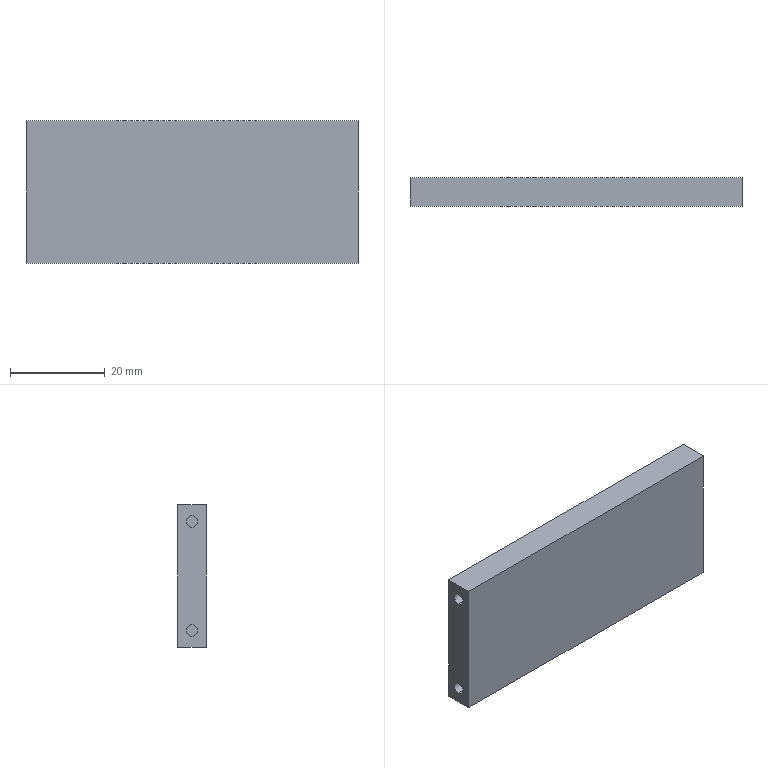Part | SolidWorks | features Cut 2, Extrusion 1 | 1 solid | 18 faces | box 70 x 6 x 30 mm | volume 12502 mm3 | plane 10 | cylinder 8 | commonest cylinder face diameters 2.5 x8
STEP:
#1=CARTESIAN_POINT('',(-30.,3.,-12.75));
#2=VERTEX_POINT('',#1);
#3=CARTESIAN_POINT('',(-30.,3.,-10.25));
#4=VERTEX_POINT('',#3);
#5=CARTESIAN_POINT('',(-30.,3.,-11.5));
#6=DIRECTION('',(-1.,0.,0.));
#7=DIRECTION('',(0.,0.,1.));
#8=AXIS2_PLACEMENT_3D('',#5,#6,#7);
#9=CIRCLE('',#8,1.25);
#10=EDGE_CURVE('',#2,#4,#9,.T.);
#11=ORIENTED_EDGE('',*,*,#10,.F.);
#12=CARTESIAN_POINT('',(-35.,3.,-12.75));
#13=VERTEX_POINT('',#12);
#14=CARTESIAN_POINT('',(-30.,3.,-12.75));
#15=DIRECTION('',(-1.,0.,0.));
#16=VECTOR('',#15,1000.);
#17=LINE('',#14,#16);
#18=EDGE_CURVE('',#2,#13,#17,.T.);
#19=ORIENTED_EDGE('',*,*,#18,.T.);
#20=CARTESIAN_POINT('',(-35.,3.,-10.25));
#21=VERTEX_POINT('',#20);
#22=CARTESIAN_POINT('',(-35.,3.,-11.5));
#23=DIRECTION('',(-1.,0.,0.));
#24=DIRECTION('',(0.,0.,1.));
#25=AXIS2_PLACEMENT_3D('',#22,#23,#24);
#26=CIRCLE('',#25,1.25);
#27=EDGE_CURVE('',#13,#21,#26,.T.);
#28=ORIENTED_EDGE('',*,*,#27,.T.);
#29=CARTESIAN_POINT('',(-30.,3.,-10.25));
#30=DIRECTION('',(-1.,0.,0.));
#31=VECTOR('',#30,1000.);
#32=LINE('',#29,#31);
#33=EDGE_CURVE('',#4,#21,#32,.T.);
#34=ORIENTED_EDGE('',*,*,#33,.F.);
#35=EDGE_LOOP('',(#11,#19,#28,#34));
#36=FACE_OUTER_BOUND('',#35,.T.);
#37=CARTESIAN_POINT('',(-30.,3.,-11.5));
#38=DIRECTION('',(-1.,0.,0.));
#39=DIRECTION('',(0.,0.,1.));
#40=AXIS2_PLACEMENT_3D('',#37,#38,#39);
#41=CYLINDRICAL_SURFACE('',#40,1.25);
#42=ADVANCED_FACE('',(#36),#41,.F.);
#43=CARTESIAN_POINT('',(-30.,3.,10.25));
#44=VERTEX_POINT('',#43);
#45=CARTESIAN_POINT('',(-30.,3.,12.75));
#46=VERTEX_POINT('',#45);
#47=CARTESIAN_POINT('',(-30.,3.,11.5));
#48=DIRECTION('',(-1.,0.,0.));
#49=DIRECTION('',(0.,0.,1.));
#50=AXIS2_PLACEMENT_3D('',#47,#48,#49);
#51=CIRCLE('',#50,1.25);
#52=EDGE_CURVE('',#44,#46,#51,.T.);
#53=ORIENTED_EDGE('',*,*,#52,.F.);
#54=CARTESIAN_POINT('',(-35.,3.,10.25));
#55=VERTEX_POINT('',#54);
#56=CARTESIAN_POINT('',(-30.,3.,10.25));
#57=DIRECTION('',(-1.,0.,0.));
#58=VECTOR('',#57,1000.);
#59=LINE('',#56,#58);
#60=EDGE_CURVE('',#44,#55,#59,.T.);
#61=ORIENTED_EDGE('',*,*,#60,.T.);
#62=CARTESIAN_POINT('',(-35.,3.,12.75));
#63=VERTEX_POINT('',#62);
#64=CARTESIAN_POINT('',(-35.,3.,11.5));
#65=DIRECTION('',(-1.,0.,0.));
#66=DIRECTION('',(0.,0.,1.));
#67=AXIS2_PLACEMENT_3D('',#64,#65,#66);
#68=CIRCLE('',#67,1.25);
#69=EDGE_CURVE('',#55,#63,#68,.T.);
#70=ORIENTED_EDGE('',*,*,#69,.T.);
#71=CARTESIAN_POINT('',(-30.,3.,12.75));
#72=DIRECTION('',(-1.,0.,0.));
#73=VECTOR('',#72,1000.);
#74=LINE('',#71,#73);
#75=EDGE_CURVE('',#46,#63,#74,.T.);
#76=ORIENTED_EDGE('',*,*,#75,.F.);
#77=EDGE_LOOP('',(#53,#61,#70,#76));
#78=FACE_OUTER_BOUND('',#77,.T.);
#79=CARTESIAN_POINT('',(-30.,3.,11.5));
#80=DIRECTION('',(-1.,0.,0.));
#81=DIRECTION('',(0.,0.,1.));
#82=AXIS2_PLACEMENT_3D('',#79,#80,#81);
#83=CYLINDRICAL_SURFACE('',#82,1.25);
#84=ADVANCED_FACE('',(#78),#83,.F.);
#85=CARTESIAN_POINT('',(30.,3.,-10.25));
#86=VERTEX_POINT('',#85);
#87=CARTESIAN_POINT('',(30.,3.,-12.75));
#88=VERTEX_POINT('',#87);
#89=CARTESIAN_POINT('',(30.,3.,-11.5));
#90=DIRECTION('',(1.,0.,0.));
#91=DIRECTION('',(0.,0.,-1.));
#92=AXIS2_PLACEMENT_3D('',#89,#90,#91);
#93=CIRCLE('',#92,1.25);
#94=EDGE_CURVE('',#86,#88,#93,.T.);
#95=ORIENTED_EDGE('',*,*,#94,.F.);
#96=CARTESIAN_POINT('',(35.,3.,-10.25));
#97=VERTEX_POINT('',#96);
#98=CARTESIAN_POINT('',(30.,3.,-10.25));
#99=DIRECTION('',(1.,0.,0.));
#100=VECTOR('',#99,1000.);
#101=LINE('',#98,#100);
#102=EDGE_CURVE('',#86,#97,#101,.T.);
#103=ORIENTED_EDGE('',*,*,#102,.T.);
#104=CARTESIAN_POINT('',(35.,3.,-12.75));
#105=VERTEX_POINT('',#104);
#106=CARTESIAN_POINT('',(35.,3.,-11.5));
#107=DIRECTION('',(1.,0.,0.));
#108=DIRECTION('',(0.,0.,-1.));
#109=AXIS2_PLACEMENT_3D('',#106,#107,#108);
#110=CIRCLE('',#109,1.25);
#111=EDGE_CURVE('',#97,#105,#110,.T.);
#112=ORIENTED_EDGE('',*,*,#111,.T.);
#113=CARTESIAN_POINT('',(30.,3.,-12.75));
#114=DIRECTION('',(1.,0.,0.));
#115=VECTOR('',#114,1000.);
#116=LINE('',#113,#115);
#117=EDGE_CURVE('',#88,#105,#116,.T.);
#118=ORIENTED_EDGE('',*,*,#117,.F.);
#119=EDGE_LOOP('',(#95,#103,#112,#118));
#120=FACE_OUTER_BOUND('',#119,.T.);
#121=CARTESIAN_POINT('',(30.,3.,-11.5));
#122=DIRECTION('',(1.,0.,0.));
#123=DIRECTION('',(0.,0.,-1.));
#124=AXIS2_PLACEMENT_3D('',#121,#122,#123);
#125=CYLINDRICAL_SURFACE('',#124,1.25);
#126=ADVANCED_FACE('',(#120),#125,.F.);
#127=CARTESIAN_POINT('',(30.,3.,12.75));
#128=VERTEX_POINT('',#127);
#129=CARTESIAN_POINT('',(30.,3.,10.25));
#130=VERTEX_POINT('',#129);
#131=CARTESIAN_POINT('',(30.,3.,11.5));
#132=DIRECTION('',(1.,0.,0.));
#133=DIRECTION('',(0.,0.,-1.));
#134=AXIS2_PLACEMENT_3D('',#131,#132,#133);
#135=CIRCLE('',#134,1.25);
#136=EDGE_CURVE('',#128,#130,#135,.T.);
#137=ORIENTED_EDGE('',*,*,#136,.F.);
#138=CARTESIAN_POINT('',(35.,3.,12.75));
#139=VERTEX_POINT('',#138);
#140=CARTESIAN_POINT('',(30.,3.,12.75));
#141=DIRECTION('',(1.,0.,0.));
#142=VECTOR('',#141,1000.);
#143=LINE('',#140,#142);
#144=EDGE_CURVE('',#128,#139,#143,.T.);
#145=ORIENTED_EDGE('',*,*,#144,.T.);
#146=CARTESIAN_POINT('',(35.,3.,10.25));
#147=VERTEX_POINT('',#146);
#148=CARTESIAN_POINT('',(35.,3.,11.5));
#149=DIRECTION('',(1.,0.,0.));
#150=DIRECTION('',(0.,0.,-1.));
#151=AXIS2_PLACEMENT_3D('',#148,#149,#150);
#152=CIRCLE('',#151,1.25);
#153=EDGE_CURVE('',#139,#147,#152,.T.);
#154=ORIENTED_EDGE('',*,*,#153,.T.);
#155=CARTESIAN_POINT('',(30.,3.,10.25));
#156=DIRECTION('',(1.,0.,0.));
#157=VECTOR('',#156,1000.);
#158=LINE('',#155,#157);
#159=EDGE_CURVE('',#130,#147,#158,.T.);
#160=ORIENTED_EDGE('',*,*,#159,.F.);
#161=EDGE_LOOP('',(#137,#145,#154,#160));
#162=FACE_OUTER_BOUND('',#161,.T.);
#163=CARTESIAN_POINT('',(30.,3.,11.5));
#164=DIRECTION('',(1.,0.,0.));
#165=DIRECTION('',(0.,0.,-1.));
#166=AXIS2_PLACEMENT_3D('',#163,#164,#165);
#167=CYLINDRICAL_SURFACE('',#166,1.25);
#168=ADVANCED_FACE('',(#162),#167,.F.);
#169=CARTESIAN_POINT('',(35.,3.,-11.5));
#170=DIRECTION('',(1.,0.,0.));
#171=DIRECTION('',(0.,0.,-1.));
#172=AXIS2_PLACEMENT_3D('',#169,#170,#171);
#173=CIRCLE('',#172,1.25);
#174=EDGE_CURVE('',#105,#97,#173,.T.);
#175=ORIENTED_EDGE('',*,*,#174,.F.);
#176=ORIENTED_EDGE('',*,*,#111,.F.);
#177=EDGE_LOOP('',(#175,#176));
#178=FACE_BOUND('',#177,.T.);
#179=CARTESIAN_POINT('',(35.,3.,11.5));
#180=DIRECTION('',(1.,0.,0.));
#181=DIRECTION('',(0.,0.,-1.));
#182=AXIS2_PLACEMENT_3D('',#179,#180,#181);
#183=CIRCLE('',#182,1.25);
#184=EDGE_CURVE('',#147,#139,#183,.T.);
#185=ORIENTED_EDGE('',*,*,#184,.F.);
#186=ORIENTED_EDGE('',*,*,#153,.F.);
#187=EDGE_LOOP('',(#185,#186));
#188=FACE_BOUND('',#187,.T.);
#189=CARTESIAN_POINT('',(35.,0.,15.));
#190=VERTEX_POINT('',#189);
#191=CARTESIAN_POINT('',(35.,0.,-15.));
#192=VERTEX_POINT('',#191);
#193=CARTESIAN_POINT('',(35.,0.,-15.));
#194=DIRECTION('',(0.,0.,-1.));
#195=VECTOR('',#194,1000.);
#196=LINE('',#193,#195);
#197=EDGE_CURVE('',#190,#192,#196,.T.);
#198=ORIENTED_EDGE('',*,*,#197,.T.);
#199=CARTESIAN_POINT('',(35.,6.,-15.));
#200=VERTEX_POINT('',#199);
#201=CARTESIAN_POINT('',(35.,6.,-15.));
#202=DIRECTION('',(0.,-1.,0.));
#203=VECTOR('',#202,1000.);
#204=LINE('',#201,#203);
#205=EDGE_CURVE('',#200,#192,#204,.T.);
#206=ORIENTED_EDGE('',*,*,#205,.F.);
#207=CARTESIAN_POINT('',(35.,6.,15.));
#208=VERTEX_POINT('',#207);
#209=CARTESIAN_POINT('',(35.,6.,-15.));
#210=DIRECTION('',(0.,0.,-1.));
#211=VECTOR('',#210,1000.);
#212=LINE('',#209,#211);
#213=EDGE_CURVE('',#208,#200,#212,.T.);
#214=ORIENTED_EDGE('',*,*,#213,.F.);
#215=CARTESIAN_POINT('',(35.,6.,15.));
#216=DIRECTION('',(0.,-1.,0.));
#217=VECTOR('',#216,1000.);
#218=LINE('',#215,#217);
#219=EDGE_CURVE('',#208,#190,#218,.T.);
#220=ORIENTED_EDGE('',*,*,#219,.T.);
#221=EDGE_LOOP('',(#198,#206,#214,#220));
#222=FACE_OUTER_BOUND('',#221,.T.);
#223=CARTESIAN_POINT('',(35.,6.,-15.));
#224=DIRECTION('',(-1.,0.,0.));
#225=DIRECTION('',(0.,0.,1.));
#226=AXIS2_PLACEMENT_3D('',#223,#224,#225);
#227=PLANE('',#226);
#228=ADVANCED_FACE('',(#178,#188,#222),#227,.F.);
#229=CARTESIAN_POINT('',(-35.,0.,-15.));
#230=VERTEX_POINT('',#229);
#231=CARTESIAN_POINT('',(-35.,0.,-15.));
#232=DIRECTION('',(-1.,0.,0.));
#233=VECTOR('',#232,1000.);
#234=LINE('',#231,#233);
#235=EDGE_CURVE('',#192,#230,#234,.T.);
#236=ORIENTED_EDGE('',*,*,#235,.T.);
#237=CARTESIAN_POINT('',(-35.,6.,-15.));
#238=VERTEX_POINT('',#237);
#239=CARTESIAN_POINT('',(-35.,6.,-15.));
#240=DIRECTION('',(0.,-1.,0.));
#241=VECTOR('',#240,1000.);
#242=LINE('',#239,#241);
#243=EDGE_CURVE('',#238,#230,#242,.T.);
#244=ORIENTED_EDGE('',*,*,#243,.F.);
#245=CARTESIAN_POINT('',(-35.,6.,-15.));
#246=DIRECTION('',(-1.,0.,0.));
#247=VECTOR('',#246,1000.);
#248=LINE('',#245,#247);
#249=EDGE_CURVE('',#200,#238,#248,.T.);
#250=ORIENTED_EDGE('',*,*,#249,.F.);
#251=ORIENTED_EDGE('',*,*,#205,.T.);
#252=EDGE_LOOP('',(#236,#244,#250,#251));
#253=FACE_OUTER_BOUND('',#252,.T.);
#254=CARTESIAN_POINT('',(-35.,6.,-15.));
#255=DIRECTION('',(0.,0.,1.));
#256=DIRECTION('',(1.,0.,0.));
#257=AXIS2_PLACEMENT_3D('',#254,#255,#256);
#258=PLANE('',#257);
#259=ADVANCED_FACE('',(#253),#258,.F.);
#260=CARTESIAN_POINT('',(-35.,3.,-11.5));
#261=DIRECTION('',(-1.,0.,0.));
#262=DIRECTION('',(0.,0.,1.));
#263=AXIS2_PLACEMENT_3D('',#260,#261,#262);
#264=CIRCLE('',#263,1.25);
#265=EDGE_CURVE('',#21,#13,#264,.T.);
#266=ORIENTED_EDGE('',*,*,#265,.F.);
#267=ORIENTED_EDGE('',*,*,#27,.F.);
#268=EDGE_LOOP('',(#266,#267));
#269=FACE_BOUND('',#268,.T.);
#270=CARTESIAN_POINT('',(-35.,3.,11.5));
#271=DIRECTION('',(-1.,0.,0.));
#272=DIRECTION('',(0.,0.,1.));
#273=AXIS2_PLACEMENT_3D('',#270,#271,#272);
#274=CIRCLE('',#273,1.25);
#275=EDGE_CURVE('',#63,#55,#274,.T.);
#276=ORIENTED_EDGE('',*,*,#275,.F.);
#277=ORIENTED_EDGE('',*,*,#69,.F.);
#278=EDGE_LOOP('',(#276,#277));
#279=FACE_BOUND('',#278,.T.);
#280=CARTESIAN_POINT('',(-35.,0.,15.));
#281=VERTEX_POINT('',#280);
#282=CARTESIAN_POINT('',(-35.,0.,-15.));
#283=DIRECTION('',(0.,0.,1.));
#284=VECTOR('',#283,1000.);
#285=LINE('',#282,#284);
#286=EDGE_CURVE('',#230,#281,#285,.T.);
#287=ORIENTED_EDGE('',*,*,#286,.T.);
#288=CARTESIAN_POINT('',(-35.,6.,15.));
#289=VERTEX_POINT('',#288);
#290=CARTESIAN_POINT('',(-35.,6.,15.));
#291=DIRECTION('',(0.,-1.,0.));
#292=VECTOR('',#291,1000.);
#293=LINE('',#290,#292);
#294=EDGE_CURVE('',#289,#281,#293,.T.);
#295=ORIENTED_EDGE('',*,*,#294,.F.);
#296=CARTESIAN_POINT('',(-35.,6.,-15.));
#297=DIRECTION('',(0.,0.,1.));
#298=VECTOR('',#297,1000.);
#299=LINE('',#296,#298);
#300=EDGE_CURVE('',#238,#289,#299,.T.);
#301=ORIENTED_EDGE('',*,*,#300,.F.);
#302=ORIENTED_EDGE('',*,*,#243,.T.);
#303=EDGE_LOOP('',(#287,#295,#301,#302));
#304=FACE_OUTER_BOUND('',#303,.T.);
#305=CARTESIAN_POINT('',(-35.,6.,-15.));
#306=DIRECTION('',(1.,0.,0.));
#307=DIRECTION('',(0.,0.,-1.));
#308=AXIS2_PLACEMENT_3D('',#305,#306,#307);
#309=PLANE('',#308);
#310=ADVANCED_FACE('',(#269,#279,#304),#309,.F.);
#311=CARTESIAN_POINT('',(-35.,0.,15.));
#312=DIRECTION('',(1.,0.,0.));
#313=VECTOR('',#312,1000.);
#314=LINE('',#311,#313);
#315=EDGE_CURVE('',#281,#190,#314,.T.);
#316=ORIENTED_EDGE('',*,*,#315,.T.);
#317=ORIENTED_EDGE('',*,*,#219,.F.);
#318=CARTESIAN_POINT('',(-35.,6.,15.));
#319=DIRECTION('',(1.,0.,0.));
#320=VECTOR('',#319,1000.);
#321=LINE('',#318,#320);
#322=EDGE_CURVE('',#289,#208,#321,.T.);
#323=ORIENTED_EDGE('',*,*,#322,.F.);
#324=ORIENTED_EDGE('',*,*,#294,.T.);
#325=EDGE_LOOP('',(#316,#317,#323,#324));
#326=FACE_OUTER_BOUND('',#325,.T.);
#327=CARTESIAN_POINT('',(-35.,6.,15.));
#328=DIRECTION('',(0.,0.,-1.));
#329=DIRECTION('',(-1.,0.,0.));
#330=AXIS2_PLACEMENT_3D('',#327,#328,#329);
#331=PLANE('',#330);
#332=ADVANCED_FACE('',(#326),#331,.F.);
#333=ORIENTED_EDGE('',*,*,#213,.T.);
#334=ORIENTED_EDGE('',*,*,#249,.T.);
#335=ORIENTED_EDGE('',*,*,#300,.T.);
#336=ORIENTED_EDGE('',*,*,#322,.T.);
#337=EDGE_LOOP('',(#333,#334,#335,#336));
#338=FACE_OUTER_BOUND('',#337,.T.);
#339=CARTESIAN_POINT('',(0.,6.,0.));
#340=DIRECTION('',(0.,1.,0.));
#341=DIRECTION('',(0.,0.,1.));
#342=AXIS2_PLACEMENT_3D('',#339,#340,#341);
#343=PLANE('',#342);
#344=ADVANCED_FACE('',(#338),#343,.T.);
#345=ORIENTED_EDGE('',*,*,#197,.F.);
#346=ORIENTED_EDGE('',*,*,#315,.F.);
#347=ORIENTED_EDGE('',*,*,#286,.F.);
#348=ORIENTED_EDGE('',*,*,#235,.F.);
#349=EDGE_LOOP('',(#345,#346,#347,#348));
#350=FACE_OUTER_BOUND('',#349,.T.);
#351=CARTESIAN_POINT('',(0.,0.,0.));
#352=DIRECTION('',(0.,1.,0.));
#353=DIRECTION('',(0.,0.,1.));
#354=AXIS2_PLACEMENT_3D('',#351,#352,#353);
#355=PLANE('',#354);
#356=ADVANCED_FACE('',(#350),#355,.F.);
#357=ORIENTED_EDGE('',*,*,#144,.F.);
#358=CARTESIAN_POINT('',(30.,3.,11.5));
#359=DIRECTION('',(1.,0.,0.));
#360=DIRECTION('',(0.,0.,-1.));
#361=AXIS2_PLACEMENT_3D('',#358,#359,#360);
#362=CIRCLE('',#361,1.25);
#363=EDGE_CURVE('',#130,#128,#362,.T.);
#364=ORIENTED_EDGE('',*,*,#363,.F.);
#365=ORIENTED_EDGE('',*,*,#159,.T.);
#366=ORIENTED_EDGE('',*,*,#184,.T.);
#367=EDGE_LOOP('',(#357,#364,#365,#366));
#368=FACE_OUTER_BOUND('',#367,.T.);
#369=CARTESIAN_POINT('',(30.,3.,11.5));
#370=DIRECTION('',(1.,0.,0.));
#371=DIRECTION('',(0.,0.,-1.));
#372=AXIS2_PLACEMENT_3D('',#369,#370,#371);
#373=CYLINDRICAL_SURFACE('',#372,1.25);
#374=ADVANCED_FACE('',(#368),#373,.F.);
#375=ORIENTED_EDGE('',*,*,#363,.T.);
#376=ORIENTED_EDGE('',*,*,#136,.T.);
#377=EDGE_LOOP('',(#375,#376));
#378=FACE_OUTER_BOUND('',#377,.T.);
#379=CARTESIAN_POINT('',(30.,3.,11.5));
#380=DIRECTION('',(1.,0.,0.));
#381=DIRECTION('',(0.,0.,-1.));
#382=AXIS2_PLACEMENT_3D('',#379,#380,#381);
#383=PLANE('',#382);
#384=ADVANCED_FACE('',(#378),#383,.T.);
#385=ORIENTED_EDGE('',*,*,#102,.F.);
#386=CARTESIAN_POINT('',(30.,3.,-11.5));
#387=DIRECTION('',(1.,0.,0.));
#388=DIRECTION('',(0.,0.,-1.));
#389=AXIS2_PLACEMENT_3D('',#386,#387,#388);
#390=CIRCLE('',#389,1.25);
#391=EDGE_CURVE('',#88,#86,#390,.T.);
#392=ORIENTED_EDGE('',*,*,#391,.F.);
#393=ORIENTED_EDGE('',*,*,#117,.T.);
#394=ORIENTED_EDGE('',*,*,#174,.T.);
#395=EDGE_LOOP('',(#385,#392,#393,#394));
#396=FACE_OUTER_BOUND('',#395,.T.);
#397=CARTESIAN_POINT('',(30.,3.,-11.5));
#398=DIRECTION('',(1.,0.,0.));
#399=DIRECTION('',(0.,0.,-1.));
#400=AXIS2_PLACEMENT_3D('',#397,#398,#399);
#401=CYLINDRICAL_SURFACE('',#400,1.25);
#402=ADVANCED_FACE('',(#396),#401,.F.);
#403=ORIENTED_EDGE('',*,*,#391,.T.);
#404=ORIENTED_EDGE('',*,*,#94,.T.);
#405=EDGE_LOOP('',(#403,#404));
#406=FACE_OUTER_BOUND('',#405,.T.);
#407=CARTESIAN_POINT('',(30.,3.,-11.5));
#408=DIRECTION('',(1.,0.,0.));
#409=DIRECTION('',(0.,0.,-1.));
#410=AXIS2_PLACEMENT_3D('',#407,#408,#409);
#411=PLANE('',#410);
#412=ADVANCED_FACE('',(#406),#411,.T.);
#413=ORIENTED_EDGE('',*,*,#60,.F.);
#414=CARTESIAN_POINT('',(-30.,3.,11.5));
#415=DIRECTION('',(-1.,0.,0.));
#416=DIRECTION('',(0.,0.,1.));
#417=AXIS2_PLACEMENT_3D('',#414,#415,#416);
#418=CIRCLE('',#417,1.25);
#419=EDGE_CURVE('',#46,#44,#418,.T.);
#420=ORIENTED_EDGE('',*,*,#419,.F.);
#421=ORIENTED_EDGE('',*,*,#75,.T.);
#422=ORIENTED_EDGE('',*,*,#275,.T.);
#423=EDGE_LOOP('',(#413,#420,#421,#422));
#424=FACE_OUTER_BOUND('',#423,.T.);
#425=CARTESIAN_POINT('',(-30.,3.,11.5));
#426=DIRECTION('',(-1.,0.,0.));
#427=DIRECTION('',(0.,0.,1.));
#428=AXIS2_PLACEMENT_3D('',#425,#426,#427);
#429=CYLINDRICAL_SURFACE('',#428,1.25);
#430=ADVANCED_FACE('',(#424),#429,.F.);
#431=ORIENTED_EDGE('',*,*,#419,.T.);
#432=ORIENTED_EDGE('',*,*,#52,.T.);
#433=EDGE_LOOP('',(#431,#432));
#434=FACE_OUTER_BOUND('',#433,.T.);
#435=CARTESIAN_POINT('',(-30.,3.,11.5));
#436=DIRECTION('',(-1.,0.,0.));
#437=DIRECTION('',(0.,0.,1.));
#438=AXIS2_PLACEMENT_3D('',#435,#436,#437);
#439=PLANE('',#438);
#440=ADVANCED_FACE('',(#434),#439,.T.);
#441=ORIENTED_EDGE('',*,*,#18,.F.);
#442=CARTESIAN_POINT('',(-30.,3.,-11.5));
#443=DIRECTION('',(-1.,0.,0.));
#444=DIRECTION('',(0.,0.,1.));
#445=AXIS2_PLACEMENT_3D('',#442,#443,#444);
#446=CIRCLE('',#445,1.25);
#447=EDGE_CURVE('',#4,#2,#446,.T.);
#448=ORIENTED_EDGE('',*,*,#447,.F.);
#449=ORIENTED_EDGE('',*,*,#33,.T.);
#450=ORIENTED_EDGE('',*,*,#265,.T.);
#451=EDGE_LOOP('',(#441,#448,#449,#450));
#452=FACE_OUTER_BOUND('',#451,.T.);
#453=CARTESIAN_POINT('',(-30.,3.,-11.5));
#454=DIRECTION('',(-1.,0.,0.));
#455=DIRECTION('',(0.,0.,1.));
#456=AXIS2_PLACEMENT_3D('',#453,#454,#455);
#457=CYLINDRICAL_SURFACE('',#456,1.25);
#458=ADVANCED_FACE('',(#452),#457,.F.);
#459=ORIENTED_EDGE('',*,*,#447,.T.);
#460=ORIENTED_EDGE('',*,*,#10,.T.);
#461=EDGE_LOOP('',(#459,#460));
#462=FACE_OUTER_BOUND('',#461,.T.);
#463=CARTESIAN_POINT('',(-30.,3.,-11.5));
#464=DIRECTION('',(-1.,0.,0.));
#465=DIRECTION('',(0.,0.,1.));
#466=AXIS2_PLACEMENT_3D('',#463,#464,#465);
#467=PLANE('',#466);
#468=ADVANCED_FACE('',(#462),#467,.T.);
#469=CLOSED_SHELL('',(#42,#84,#126,#168,#228,#259,#310,#332,#344,#356,#374,#384,#402,#412,#430,#440,#458,#468));
#470=MANIFOLD_SOLID_BREP('',#469);
#471=CARTESIAN_POINT('',(0.,0.,0.));
#472=DIRECTION('',(0.,0.,1.));
#473=DIRECTION('',(1.,0.,0.));
#474=AXIS2_PLACEMENT_3D('',#471,#472,#473);
#475=(LENGTH_UNIT()NAMED_UNIT(*)SI_UNIT(.MILLI.,.METRE.));
#476=UNCERTAINTY_MEASURE_WITH_UNIT(LENGTH_MEASURE(0.00001),#475,'','');
#477=(NAMED_UNIT(*)PLANE_ANGLE_UNIT()SI_UNIT($,.RADIAN.));
#478=(NAMED_UNIT(*)SI_UNIT($,.STERADIAN.)SOLID_ANGLE_UNIT());
#479=(GEOMETRIC_REPRESENTATION_CONTEXT(3)GLOBAL_UNCERTAINTY_ASSIGNED_CONTEXT((#476))GLOBAL_UNIT_ASSIGNED_CONTEXT((#475,#477,#478))REPRESENTATION_CONTEXT('',''));
#480=ADVANCED_BREP_SHAPE_REPRESENTATION('',(#470,#474),#479);